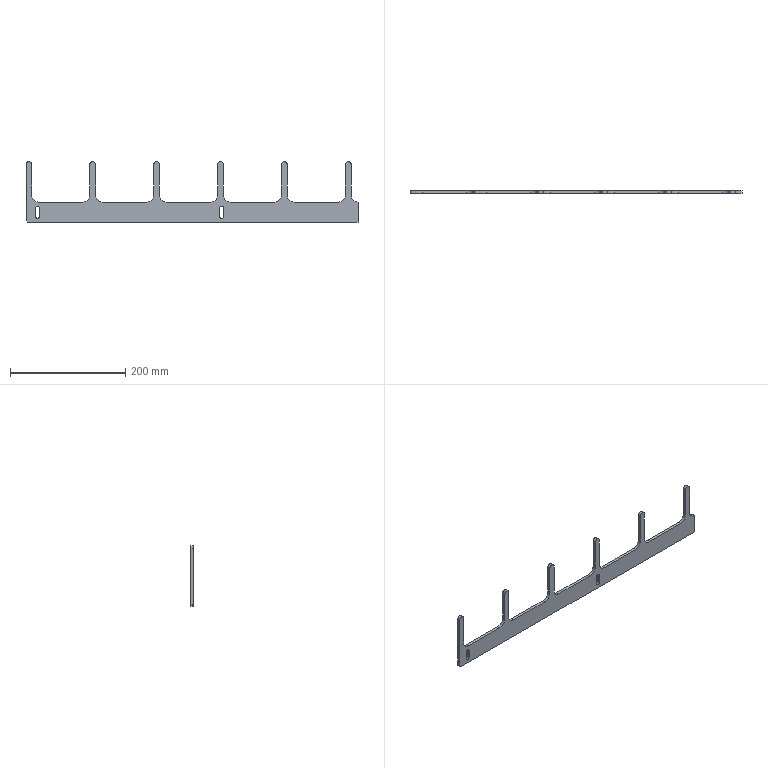Part | SolidWorks | features BaseBody 1, ICE 1 | 1 solid | 47 faces | box 577 x 5 x 105 mm | volume 122030 mm3 | plane 26 | cylinder 21 | commonest cylinder face diameters 24 x11 10 x6 6.5 x4
STEP:
#1=CARTESIAN_POINT('',(17.,0.,-5.));
#2=VERTEX_POINT('',#1);
#3=CARTESIAN_POINT('',(17.,0.,30.));
#4=VERTEX_POINT('',#3);
#5=CARTESIAN_POINT('',(17.,0.,47.5));
#6=DIRECTION('',(0.,0.,1.));
#7=VECTOR('',#6,1000.);
#8=LINE('',#5,#7);
#9=EDGE_CURVE('',#2,#4,#8,.T.);
#10=ORIENTED_EDGE('',*,*,#9,.F.);
#11=CARTESIAN_POINT('',(-557.5,0.,-5.));
#12=VERTEX_POINT('',#11);
#13=CARTESIAN_POINT('',(-557.5,0.,-5.));
#14=DIRECTION('',(1.,0.,0.));
#15=VECTOR('',#14,1000.);
#16=LINE('',#13,#15);
#17=EDGE_CURVE('',#12,#2,#16,.T.);
#18=ORIENTED_EDGE('',*,*,#17,.F.);
#19=CARTESIAN_POINT('',(-560.,0.,-2.5));
#20=VERTEX_POINT('',#19);
#21=CARTESIAN_POINT('',(-560.,0.,-2.5));
#22=DIRECTION('',(0.7071,0.,-0.7071));
#23=VECTOR('',#22,1000.);
#24=LINE('',#21,#23);
#25=EDGE_CURVE('',#20,#12,#24,.T.);
#26=ORIENTED_EDGE('',*,*,#25,.F.);
#27=CARTESIAN_POINT('',(-560.,0.,95.));
#28=VERTEX_POINT('',#27);
#29=CARTESIAN_POINT('',(-560.,0.,95.));
#30=DIRECTION('',(0.,0.,-1.));
#31=VECTOR('',#30,1000.);
#32=LINE('',#29,#31);
#33=EDGE_CURVE('',#28,#20,#32,.T.);
#34=ORIENTED_EDGE('',*,*,#33,.F.);
#35=CARTESIAN_POINT('',(-550.,0.,95.));
#36=VERTEX_POINT('',#35);
#37=CARTESIAN_POINT('',(-555.,0.,95.));
#38=DIRECTION('',(0.,-1.,0.));
#39=DIRECTION('',(1.,0.,0.));
#40=AXIS2_PLACEMENT_3D('',#37,#38,#39);
#41=CIRCLE('',#40,5.);
#42=EDGE_CURVE('',#36,#28,#41,.T.);
#43=ORIENTED_EDGE('',*,*,#42,.F.);
#44=CARTESIAN_POINT('',(-550.,0.,42.));
#45=VERTEX_POINT('',#44);
#46=CARTESIAN_POINT('',(-550.,0.,42.));
#47=DIRECTION('',(0.,0.,1.));
#48=VECTOR('',#47,1000.);
#49=LINE('',#46,#48);
#50=EDGE_CURVE('',#45,#36,#49,.T.);
#51=ORIENTED_EDGE('',*,*,#50,.F.);
#52=CARTESIAN_POINT('',(-538.,0.,30.));
#53=VERTEX_POINT('',#52);
#54=CARTESIAN_POINT('',(-538.,0.,42.));
#55=DIRECTION('',(0.,1.,0.));
#56=DIRECTION('',(0.,0.,-1.));
#57=AXIS2_PLACEMENT_3D('',#54,#55,#56);
#58=CIRCLE('',#57,12.);
#59=EDGE_CURVE('',#53,#45,#58,.T.);
#60=ORIENTED_EDGE('',*,*,#59,.F.);
#61=CARTESIAN_POINT('',(-461.,0.,30.));
#62=VERTEX_POINT('',#61);
#63=CARTESIAN_POINT('',(-461.,0.,30.));
#64=DIRECTION('',(-1.,0.,0.));
#65=VECTOR('',#64,1000.);
#66=LINE('',#63,#65);
#67=EDGE_CURVE('',#62,#53,#66,.T.);
#68=ORIENTED_EDGE('',*,*,#67,.F.);
#69=CARTESIAN_POINT('',(-449.,0.,42.));
#70=VERTEX_POINT('',#69);
#71=CARTESIAN_POINT('',(-461.,0.,42.));
#72=DIRECTION('',(0.,1.,0.));
#73=DIRECTION('',(1.,0.,0.));
#74=AXIS2_PLACEMENT_3D('',#71,#72,#73);
#75=CIRCLE('',#74,12.);
#76=EDGE_CURVE('',#70,#62,#75,.T.);
#77=ORIENTED_EDGE('',*,*,#76,.F.);
#78=CARTESIAN_POINT('',(-449.,0.,95.));
#79=VERTEX_POINT('',#78);
#80=CARTESIAN_POINT('',(-449.,0.,95.));
#81=DIRECTION('',(0.,0.,-1.));
#82=VECTOR('',#81,1000.);
#83=LINE('',#80,#82);
#84=EDGE_CURVE('',#79,#70,#83,.T.);
#85=ORIENTED_EDGE('',*,*,#84,.F.);
#86=CARTESIAN_POINT('',(-439.,0.,95.));
#87=VERTEX_POINT('',#86);
#88=CARTESIAN_POINT('',(-444.,0.,95.));
#89=DIRECTION('',(0.,-1.,0.));
#90=DIRECTION('',(1.,0.,0.));
#91=AXIS2_PLACEMENT_3D('',#88,#89,#90);
#92=CIRCLE('',#91,5.);
#93=EDGE_CURVE('',#87,#79,#92,.T.);
#94=ORIENTED_EDGE('',*,*,#93,.F.);
#95=CARTESIAN_POINT('',(-439.,0.,42.));
#96=VERTEX_POINT('',#95);
#97=CARTESIAN_POINT('',(-439.,0.,42.));
#98=DIRECTION('',(0.,0.,1.));
#99=VECTOR('',#98,1000.);
#100=LINE('',#97,#99);
#101=EDGE_CURVE('',#96,#87,#100,.T.);
#102=ORIENTED_EDGE('',*,*,#101,.F.);
#103=CARTESIAN_POINT('',(-427.,0.,30.));
#104=VERTEX_POINT('',#103);
#105=CARTESIAN_POINT('',(-427.,0.,42.));
#106=DIRECTION('',(0.,1.,0.));
#107=DIRECTION('',(0.,0.,-1.));
#108=AXIS2_PLACEMENT_3D('',#105,#106,#107);
#109=CIRCLE('',#108,12.);
#110=EDGE_CURVE('',#104,#96,#109,.T.);
#111=ORIENTED_EDGE('',*,*,#110,.F.);
#112=CARTESIAN_POINT('',(-350.,0.,30.));
#113=VERTEX_POINT('',#112);
#114=CARTESIAN_POINT('',(-350.,0.,30.));
#115=DIRECTION('',(-1.,0.,0.));
#116=VECTOR('',#115,1000.);
#117=LINE('',#114,#116);
#118=EDGE_CURVE('',#113,#104,#117,.T.);
#119=ORIENTED_EDGE('',*,*,#118,.F.);
#120=CARTESIAN_POINT('',(-338.,0.,42.));
#121=VERTEX_POINT('',#120);
#122=CARTESIAN_POINT('',(-350.,0.,42.));
#123=DIRECTION('',(0.,1.,0.));
#124=DIRECTION('',(1.,0.,0.));
#125=AXIS2_PLACEMENT_3D('',#122,#123,#124);
#126=CIRCLE('',#125,12.);
#127=EDGE_CURVE('',#121,#113,#126,.T.);
#128=ORIENTED_EDGE('',*,*,#127,.F.);
#129=CARTESIAN_POINT('',(-338.,0.,95.));
#130=VERTEX_POINT('',#129);
#131=CARTESIAN_POINT('',(-338.,0.,95.));
#132=DIRECTION('',(0.,0.,-1.));
#133=VECTOR('',#132,1000.);
#134=LINE('',#131,#133);
#135=EDGE_CURVE('',#130,#121,#134,.T.);
#136=ORIENTED_EDGE('',*,*,#135,.F.);
#137=CARTESIAN_POINT('',(-328.,0.,95.));
#138=VERTEX_POINT('',#137);
#139=CARTESIAN_POINT('',(-333.,0.,95.));
#140=DIRECTION('',(0.,-1.,0.));
#141=DIRECTION('',(1.,0.,0.));
#142=AXIS2_PLACEMENT_3D('',#139,#140,#141);
#143=CIRCLE('',#142,5.);
#144=EDGE_CURVE('',#138,#130,#143,.T.);
#145=ORIENTED_EDGE('',*,*,#144,.F.);
#146=CARTESIAN_POINT('',(-328.,0.,42.));
#147=VERTEX_POINT('',#146);
#148=CARTESIAN_POINT('',(-328.,0.,42.));
#149=DIRECTION('',(0.,0.,1.));
#150=VECTOR('',#149,1000.);
#151=LINE('',#148,#150);
#152=EDGE_CURVE('',#147,#138,#151,.T.);
#153=ORIENTED_EDGE('',*,*,#152,.F.);
#154=CARTESIAN_POINT('',(-316.,0.,30.));
#155=VERTEX_POINT('',#154);
#156=CARTESIAN_POINT('',(-316.,0.,42.));
#157=DIRECTION('',(0.,1.,0.));
#158=DIRECTION('',(0.,0.,-1.));
#159=AXIS2_PLACEMENT_3D('',#156,#157,#158);
#160=CIRCLE('',#159,12.);
#161=EDGE_CURVE('',#155,#147,#160,.T.);
#162=ORIENTED_EDGE('',*,*,#161,.F.);
#163=CARTESIAN_POINT('',(-239.,0.,30.));
#164=VERTEX_POINT('',#163);
#165=CARTESIAN_POINT('',(-239.,0.,30.));
#166=DIRECTION('',(-1.,0.,0.));
#167=VECTOR('',#166,1000.);
#168=LINE('',#165,#167);
#169=EDGE_CURVE('',#164,#155,#168,.T.);
#170=ORIENTED_EDGE('',*,*,#169,.F.);
#171=CARTESIAN_POINT('',(-227.,0.,42.));
#172=VERTEX_POINT('',#171);
#173=CARTESIAN_POINT('',(-239.,0.,42.));
#174=DIRECTION('',(0.,1.,0.));
#175=DIRECTION('',(1.,0.,0.));
#176=AXIS2_PLACEMENT_3D('',#173,#174,#175);
#177=CIRCLE('',#176,12.);
#178=EDGE_CURVE('',#172,#164,#177,.T.);
#179=ORIENTED_EDGE('',*,*,#178,.F.);
#180=CARTESIAN_POINT('',(-227.,0.,95.));
#181=VERTEX_POINT('',#180);
#182=CARTESIAN_POINT('',(-227.,0.,95.));
#183=DIRECTION('',(0.,0.,-1.));
#184=VECTOR('',#183,1000.);
#185=LINE('',#182,#184);
#186=EDGE_CURVE('',#181,#172,#185,.T.);
#187=ORIENTED_EDGE('',*,*,#186,.F.);
#188=CARTESIAN_POINT('',(-217.,0.,95.));
#189=VERTEX_POINT('',#188);
#190=CARTESIAN_POINT('',(-222.,0.,95.));
#191=DIRECTION('',(0.,-1.,0.));
#192=DIRECTION('',(1.,0.,0.));
#193=AXIS2_PLACEMENT_3D('',#190,#191,#192);
#194=CIRCLE('',#193,5.);
#195=EDGE_CURVE('',#189,#181,#194,.T.);
#196=ORIENTED_EDGE('',*,*,#195,.F.);
#197=CARTESIAN_POINT('',(-217.,0.,42.));
#198=VERTEX_POINT('',#197);
#199=CARTESIAN_POINT('',(-217.,0.,42.));
#200=DIRECTION('',(0.,0.,1.));
#201=VECTOR('',#200,1000.);
#202=LINE('',#199,#201);
#203=EDGE_CURVE('',#198,#189,#202,.T.);
#204=ORIENTED_EDGE('',*,*,#203,.F.);
#205=CARTESIAN_POINT('',(-205.,0.,30.));
#206=VERTEX_POINT('',#205);
#207=CARTESIAN_POINT('',(-205.,0.,42.));
#208=DIRECTION('',(0.,1.,0.));
#209=DIRECTION('',(0.,0.,-1.));
#210=AXIS2_PLACEMENT_3D('',#207,#208,#209);
#211=CIRCLE('',#210,12.);
#212=EDGE_CURVE('',#206,#198,#211,.T.);
#213=ORIENTED_EDGE('',*,*,#212,.F.);
#214=CARTESIAN_POINT('',(-128.,0.,30.));
#215=VERTEX_POINT('',#214);
#216=CARTESIAN_POINT('',(-128.,0.,30.));
#217=DIRECTION('',(-1.,0.,0.));
#218=VECTOR('',#217,1000.);
#219=LINE('',#216,#218);
#220=EDGE_CURVE('',#215,#206,#219,.T.);
#221=ORIENTED_EDGE('',*,*,#220,.F.);
#222=CARTESIAN_POINT('',(-116.,0.,42.));
#223=VERTEX_POINT('',#222);
#224=CARTESIAN_POINT('',(-128.,0.,42.));
#225=DIRECTION('',(0.,1.,0.));
#226=DIRECTION('',(1.,0.,0.));
#227=AXIS2_PLACEMENT_3D('',#224,#225,#226);
#228=CIRCLE('',#227,12.);
#229=EDGE_CURVE('',#223,#215,#228,.T.);
#230=ORIENTED_EDGE('',*,*,#229,.F.);
#231=CARTESIAN_POINT('',(-116.,0.,95.));
#232=VERTEX_POINT('',#231);
#233=CARTESIAN_POINT('',(-116.,0.,95.));
#234=DIRECTION('',(0.,0.,-1.));
#235=VECTOR('',#234,1000.);
#236=LINE('',#233,#235);
#237=EDGE_CURVE('',#232,#223,#236,.T.);
#238=ORIENTED_EDGE('',*,*,#237,.F.);
#239=CARTESIAN_POINT('',(-106.,0.,95.));
#240=VERTEX_POINT('',#239);
#241=CARTESIAN_POINT('',(-111.,0.,95.));
#242=DIRECTION('',(0.,-1.,0.));
#243=DIRECTION('',(1.,0.,0.));
#244=AXIS2_PLACEMENT_3D('',#241,#242,#243);
#245=CIRCLE('',#244,5.);
#246=EDGE_CURVE('',#240,#232,#245,.T.);
#247=ORIENTED_EDGE('',*,*,#246,.F.);
#248=CARTESIAN_POINT('',(-106.,0.,42.));
#249=VERTEX_POINT('',#248);
#250=CARTESIAN_POINT('',(-106.,0.,42.));
#251=DIRECTION('',(0.,0.,1.));
#252=VECTOR('',#251,1000.);
#253=LINE('',#250,#252);
#254=EDGE_CURVE('',#249,#240,#253,.T.);
#255=ORIENTED_EDGE('',*,*,#254,.F.);
#256=CARTESIAN_POINT('',(-94.,0.,30.));
#257=VERTEX_POINT('',#256);
#258=CARTESIAN_POINT('',(-94.,0.,42.));
#259=DIRECTION('',(0.,1.,0.));
#260=DIRECTION('',(0.,0.,-1.));
#261=AXIS2_PLACEMENT_3D('',#258,#259,#260);
#262=CIRCLE('',#261,12.);
#263=EDGE_CURVE('',#257,#249,#262,.T.);
#264=ORIENTED_EDGE('',*,*,#263,.F.);
#265=CARTESIAN_POINT('',(-17.,0.,30.));
#266=VERTEX_POINT('',#265);
#267=CARTESIAN_POINT('',(-17.,0.,30.));
#268=DIRECTION('',(-1.,0.,0.));
#269=VECTOR('',#268,1000.);
#270=LINE('',#267,#269);
#271=EDGE_CURVE('',#266,#257,#270,.T.);
#272=ORIENTED_EDGE('',*,*,#271,.F.);
#273=CARTESIAN_POINT('',(-5.,0.,42.));
#274=VERTEX_POINT('',#273);
#275=CARTESIAN_POINT('',(-17.,0.,42.));
#276=DIRECTION('',(0.,1.,0.));
#277=DIRECTION('',(1.,0.,0.));
#278=AXIS2_PLACEMENT_3D('',#275,#276,#277);
#279=CIRCLE('',#278,12.);
#280=EDGE_CURVE('',#274,#266,#279,.T.);
#281=ORIENTED_EDGE('',*,*,#280,.F.);
#282=CARTESIAN_POINT('',(-5.,0.,95.));
#283=VERTEX_POINT('',#282);
#284=CARTESIAN_POINT('',(-5.,0.,95.));
#285=DIRECTION('',(0.,0.,-1.));
#286=VECTOR('',#285,1000.);
#287=LINE('',#284,#286);
#288=EDGE_CURVE('',#283,#274,#287,.T.);
#289=ORIENTED_EDGE('',*,*,#288,.F.);
#290=CARTESIAN_POINT('',(5.,0.,95.));
#291=VERTEX_POINT('',#290);
#292=CARTESIAN_POINT('',(0.,0.,95.));
#293=DIRECTION('',(0.,-1.,0.));
#294=DIRECTION('',(1.,0.,0.));
#295=AXIS2_PLACEMENT_3D('',#292,#293,#294);
#296=CIRCLE('',#295,5.);
#297=EDGE_CURVE('',#291,#283,#296,.T.);
#298=ORIENTED_EDGE('',*,*,#297,.F.);
#299=CARTESIAN_POINT('',(5.,0.,42.));
#300=VERTEX_POINT('',#299);
#301=CARTESIAN_POINT('',(5.,0.,42.));
#302=DIRECTION('',(0.,0.,1.));
#303=VECTOR('',#302,1000.);
#304=LINE('',#301,#303);
#305=EDGE_CURVE('',#300,#291,#304,.T.);
#306=ORIENTED_EDGE('',*,*,#305,.F.);
#307=CARTESIAN_POINT('',(17.,0.,42.));
#308=DIRECTION('',(0.,1.,0.));
#309=DIRECTION('',(0.,0.,-1.));
#310=AXIS2_PLACEMENT_3D('',#307,#308,#309);
#311=CIRCLE('',#310,12.);
#312=EDGE_CURVE('',#4,#300,#311,.T.);
#313=ORIENTED_EDGE('',*,*,#312,.F.);
#314=EDGE_LOOP('',(#10,#18,#26,#34,#43,#51,#60,#68,#77,#85,#94,#102,#111,#119,#128,#136,#145,#153,#162,#170,#179,#187,#196,#204,#213,#221,#230,#238,#247,#255,#264,#272,#281,#289,#298,#306,#313));
#315=FACE_OUTER_BOUND('',#314,.T.);
#316=CARTESIAN_POINT('',(-223.25,0.,19.5));
#317=VERTEX_POINT('',#316);
#318=CARTESIAN_POINT('',(-216.75,0.,19.5));
#319=VERTEX_POINT('',#318);
#320=CARTESIAN_POINT('',(-220.,0.,19.5));
#321=DIRECTION('',(0.,1.,0.));
#322=DIRECTION('',(-1.,0.,0.));
#323=AXIS2_PLACEMENT_3D('',#320,#321,#322);
#324=CIRCLE('',#323,3.25);
#325=EDGE_CURVE('',#317,#319,#324,.T.);
#326=ORIENTED_EDGE('',*,*,#325,.F.);
#327=CARTESIAN_POINT('',(-223.25,0.,4.5));
#328=VERTEX_POINT('',#327);
#329=CARTESIAN_POINT('',(-223.25,0.,4.5));
#330=DIRECTION('',(0.,0.,1.));
#331=VECTOR('',#330,1000.);
#332=LINE('',#329,#331);
#333=EDGE_CURVE('',#328,#317,#332,.T.);
#334=ORIENTED_EDGE('',*,*,#333,.F.);
#335=CARTESIAN_POINT('',(-216.75,0.,4.5));
#336=VERTEX_POINT('',#335);
#337=CARTESIAN_POINT('',(-220.,0.,4.5));
#338=DIRECTION('',(0.,1.,0.));
#339=DIRECTION('',(1.,0.,0.));
#340=AXIS2_PLACEMENT_3D('',#337,#338,#339);
#341=CIRCLE('',#340,3.25);
#342=EDGE_CURVE('',#336,#328,#341,.T.);
#343=ORIENTED_EDGE('',*,*,#342,.F.);
#344=CARTESIAN_POINT('',(-216.75,0.,19.5));
#345=DIRECTION('',(0.,0.,-1.));
#346=VECTOR('',#345,1000.);
#347=LINE('',#344,#346);
#348=EDGE_CURVE('',#319,#336,#347,.T.);
#349=ORIENTED_EDGE('',*,*,#348,.F.);
#350=EDGE_LOOP('',(#326,#334,#343,#349));
#351=FACE_BOUND('',#350,.T.);
#352=CARTESIAN_POINT('',(-543.25,0.,4.5));
#353=VERTEX_POINT('',#352);
#354=CARTESIAN_POINT('',(-543.25,0.,19.5));
#355=VERTEX_POINT('',#354);
#356=CARTESIAN_POINT('',(-543.25,0.,4.5));
#357=DIRECTION('',(0.,0.,1.));
#358=VECTOR('',#357,1000.);
#359=LINE('',#356,#358);
#360=EDGE_CURVE('',#353,#355,#359,.T.);
#361=ORIENTED_EDGE('',*,*,#360,.F.);
#362=CARTESIAN_POINT('',(-536.75,0.,4.5));
#363=VERTEX_POINT('',#362);
#364=CARTESIAN_POINT('',(-540.,0.,4.5));
#365=DIRECTION('',(0.,1.,0.));
#366=DIRECTION('',(1.,0.,0.));
#367=AXIS2_PLACEMENT_3D('',#364,#365,#366);
#368=CIRCLE('',#367,3.25);
#369=EDGE_CURVE('',#363,#353,#368,.T.);
#370=ORIENTED_EDGE('',*,*,#369,.F.);
#371=CARTESIAN_POINT('',(-536.75,0.,19.5));
#372=VERTEX_POINT('',#371);
#373=CARTESIAN_POINT('',(-536.75,0.,19.5));
#374=DIRECTION('',(0.,0.,-1.));
#375=VECTOR('',#374,1000.);
#376=LINE('',#373,#375);
#377=EDGE_CURVE('',#372,#363,#376,.T.);
#378=ORIENTED_EDGE('',*,*,#377,.F.);
#379=CARTESIAN_POINT('',(-540.,0.,19.5));
#380=DIRECTION('',(0.,1.,0.));
#381=DIRECTION('',(-1.,0.,0.));
#382=AXIS2_PLACEMENT_3D('',#379,#380,#381);
#383=CIRCLE('',#382,3.25);
#384=EDGE_CURVE('',#355,#372,#383,.T.);
#385=ORIENTED_EDGE('',*,*,#384,.F.);
#386=EDGE_LOOP('',(#361,#370,#378,#385));
#387=FACE_BOUND('',#386,.T.);
#388=CARTESIAN_POINT('',(0.,0.,47.5));
#389=DIRECTION('',(0.,1.,0.));
#390=DIRECTION('',(0.,0.,-1.));
#391=AXIS2_PLACEMENT_3D('',#388,#389,#390);
#392=PLANE('',#391);
#393=ADVANCED_FACE('',(#315,#351,#387),#392,.T.);
#394=CARTESIAN_POINT('',(17.,-5.,30.));
#395=VERTEX_POINT('',#394);
#396=CARTESIAN_POINT('',(17.,-5.,-5.));
#397=VERTEX_POINT('',#396);
#398=CARTESIAN_POINT('',(17.,-5.,30.));
#399=DIRECTION('',(0.,0.,-1.));
#400=VECTOR('',#399,1000.);
#401=LINE('',#398,#400);
#402=EDGE_CURVE('',#395,#397,#401,.T.);
#403=ORIENTED_EDGE('',*,*,#402,.F.);
#404=CARTESIAN_POINT('',(5.,-5.,42.));
#405=VERTEX_POINT('',#404);
#406=CARTESIAN_POINT('',(17.,-5.,42.));
#407=DIRECTION('',(0.,-1.,0.));
#408=DIRECTION('',(-1.,0.,0.));
#409=AXIS2_PLACEMENT_3D('',#406,#407,#408);
#410=CIRCLE('',#409,12.);
#411=EDGE_CURVE('',#405,#395,#410,.T.);
#412=ORIENTED_EDGE('',*,*,#411,.F.);
#413=CARTESIAN_POINT('',(5.,-5.,95.));
#414=VERTEX_POINT('',#413);
#415=CARTESIAN_POINT('',(5.,-5.,95.));
#416=DIRECTION('',(0.,0.,-1.));
#417=VECTOR('',#416,1000.);
#418=LINE('',#415,#417);
#419=EDGE_CURVE('',#414,#405,#418,.T.);
#420=ORIENTED_EDGE('',*,*,#419,.F.);
#421=CARTESIAN_POINT('',(-5.,-5.,95.));
#422=VERTEX_POINT('',#421);
#423=CARTESIAN_POINT('',(0.,-5.,95.));
#424=DIRECTION('',(0.,1.,0.));
#425=DIRECTION('',(-1.,0.,0.));
#426=AXIS2_PLACEMENT_3D('',#423,#424,#425);
#427=CIRCLE('',#426,5.);
#428=EDGE_CURVE('',#422,#414,#427,.T.);
#429=ORIENTED_EDGE('',*,*,#428,.F.);
#430=CARTESIAN_POINT('',(-5.,-5.,42.));
#431=VERTEX_POINT('',#430);
#432=CARTESIAN_POINT('',(-5.,-5.,42.));
#433=DIRECTION('',(0.,0.,1.));
#434=VECTOR('',#433,1000.);
#435=LINE('',#432,#434);
#436=EDGE_CURVE('',#431,#422,#435,.T.);
#437=ORIENTED_EDGE('',*,*,#436,.F.);
#438=CARTESIAN_POINT('',(-17.,-5.,30.));
#439=VERTEX_POINT('',#438);
#440=CARTESIAN_POINT('',(-17.,-5.,42.));
#441=DIRECTION('',(0.,-1.,0.));
#442=DIRECTION('',(0.,0.,-1.));
#443=AXIS2_PLACEMENT_3D('',#440,#441,#442);
#444=CIRCLE('',#443,12.);
#445=EDGE_CURVE('',#439,#431,#444,.T.);
#446=ORIENTED_EDGE('',*,*,#445,.F.);
#447=CARTESIAN_POINT('',(-94.,-5.,30.));
#448=VERTEX_POINT('',#447);
#449=CARTESIAN_POINT('',(-94.,-5.,30.));
#450=DIRECTION('',(1.,0.,0.));
#451=VECTOR('',#450,1000.);
#452=LINE('',#449,#451);
#453=EDGE_CURVE('',#448,#439,#452,.T.);
#454=ORIENTED_EDGE('',*,*,#453,.F.);
#455=CARTESIAN_POINT('',(-106.,-5.,42.));
#456=VERTEX_POINT('',#455);
#457=CARTESIAN_POINT('',(-94.,-5.,42.));
#458=DIRECTION('',(0.,-1.,0.));
#459=DIRECTION('',(-1.,0.,0.));
#460=AXIS2_PLACEMENT_3D('',#457,#458,#459);
#461=CIRCLE('',#460,12.);
#462=EDGE_CURVE('',#456,#448,#461,.T.);
#463=ORIENTED_EDGE('',*,*,#462,.F.);
#464=CARTESIAN_POINT('',(-106.,-5.,95.));
#465=VERTEX_POINT('',#464);
#466=CARTESIAN_POINT('',(-106.,-5.,95.));
#467=DIRECTION('',(0.,0.,-1.));
#468=VECTOR('',#467,1000.);
#469=LINE('',#466,#468);
#470=EDGE_CURVE('',#465,#456,#469,.T.);
#471=ORIENTED_EDGE('',*,*,#470,.F.);
#472=CARTESIAN_POINT('',(-116.,-5.,95.));
#473=VERTEX_POINT('',#472);
#474=CARTESIAN_POINT('',(-111.,-5.,95.));
#475=DIRECTION('',(0.,1.,0.));
#476=DIRECTION('',(-1.,0.,0.));
#477=AXIS2_PLACEMENT_3D('',#474,#475,#476);
#478=CIRCLE('',#477,5.);
#479=EDGE_CURVE('',#473,#465,#478,.T.);
#480=ORIENTED_EDGE('',*,*,#479,.F.);
#481=CARTESIAN_POINT('',(-116.,-5.,42.));
#482=VERTEX_POINT('',#481);
#483=CARTESIAN_POINT('',(-116.,-5.,42.));
#484=DIRECTION('',(0.,0.,1.));
#485=VECTOR('',#484,1000.);
#486=LINE('',#483,#485);
#487=EDGE_CURVE('',#482,#473,#486,.T.);
#488=ORIENTED_EDGE('',*,*,#487,.F.);
#489=CARTESIAN_POINT('',(-128.,-5.,30.));
#490=VERTEX_POINT('',#489);
#491=CARTESIAN_POINT('',(-128.,-5.,42.));
#492=DIRECTION('',(0.,-1.,0.));
#493=DIRECTION('',(0.,0.,-1.));
#494=AXIS2_PLACEMENT_3D('',#491,#492,#493);
#495=CIRCLE('',#494,12.);
#496=EDGE_CURVE('',#490,#482,#495,.T.);
#497=ORIENTED_EDGE('',*,*,#496,.F.);
#498=CARTESIAN_POINT('',(-205.,-5.,30.));
#499=VERTEX_POINT('',#498);
#500=CARTESIAN_POINT('',(-205.,-5.,30.));
#501=DIRECTION('',(1.,0.,0.));
#502=VECTOR('',#501,1000.);
#503=LINE('',#500,#502);
#504=EDGE_CURVE('',#499,#490,#503,.T.);
#505=ORIENTED_EDGE('',*,*,#504,.F.);
#506=CARTESIAN_POINT('',(-217.,-5.,42.));
#507=VERTEX_POINT('',#506);
#508=CARTESIAN_POINT('',(-205.,-5.,42.));
#509=DIRECTION('',(0.,-1.,0.));
#510=DIRECTION('',(-1.,0.,0.));
#511=AXIS2_PLACEMENT_3D('',#508,#509,#510);
#512=CIRCLE('',#511,12.);
#513=EDGE_CURVE('',#507,#499,#512,.T.);
#514=ORIENTED_EDGE('',*,*,#513,.F.);
#515=CARTESIAN_POINT('',(-217.,-5.,95.));
#516=VERTEX_POINT('',#515);
#517=CARTESIAN_POINT('',(-217.,-5.,95.));
#518=DIRECTION('',(0.,0.,-1.));
#519=VECTOR('',#518,1000.);
#520=LINE('',#517,#519);
#521=EDGE_CURVE('',#516,#507,#520,.T.);
#522=ORIENTED_EDGE('',*,*,#521,.F.);
#523=CARTESIAN_POINT('',(-227.,-5.,95.));
#524=VERTEX_POINT('',#523);
#525=CARTESIAN_POINT('',(-222.,-5.,95.));
#526=DIRECTION('',(0.,1.,0.));
#527=DIRECTION('',(-1.,0.,0.));
#528=AXIS2_PLACEMENT_3D('',#525,#526,#527);
#529=CIRCLE('',#528,5.);
#530=EDGE_CURVE('',#524,#516,#529,.T.);
#531=ORIENTED_EDGE('',*,*,#530,.F.);
#532=CARTESIAN_POINT('',(-227.,-5.,42.));
#533=VERTEX_POINT('',#532);
#534=CARTESIAN_POINT('',(-227.,-5.,42.));
#535=DIRECTION('',(0.,0.,1.));
#536=VECTOR('',#535,1000.);
#537=LINE('',#534,#536);
#538=EDGE_CURVE('',#533,#524,#537,.T.);
#539=ORIENTED_EDGE('',*,*,#538,.F.);
#540=CARTESIAN_POINT('',(-239.,-5.,30.));
#541=VERTEX_POINT('',#540);
#542=CARTESIAN_POINT('',(-239.,-5.,42.));
#543=DIRECTION('',(0.,-1.,0.));
#544=DIRECTION('',(0.,0.,-1.));
#545=AXIS2_PLACEMENT_3D('',#542,#543,#544);
#546=CIRCLE('',#545,12.);
#547=EDGE_CURVE('',#541,#533,#546,.T.);
#548=ORIENTED_EDGE('',*,*,#547,.F.);
#549=CARTESIAN_POINT('',(-316.,-5.,30.));
#550=VERTEX_POINT('',#549);
#551=CARTESIAN_POINT('',(-316.,-5.,30.));
#552=DIRECTION('',(1.,0.,0.));
#553=VECTOR('',#552,1000.);
#554=LINE('',#551,#553);
#555=EDGE_CURVE('',#550,#541,#554,.T.);
#556=ORIENTED_EDGE('',*,*,#555,.F.);
#557=CARTESIAN_POINT('',(-328.,-5.,42.));
#558=VERTEX_POINT('',#557);
#559=CARTESIAN_POINT('',(-316.,-5.,42.));
#560=DIRECTION('',(0.,-1.,0.));
#561=DIRECTION('',(-1.,0.,0.));
#562=AXIS2_PLACEMENT_3D('',#559,#560,#561);
#563=CIRCLE('',#562,12.);
#564=EDGE_CURVE('',#558,#550,#563,.T.);
#565=ORIENTED_EDGE('',*,*,#564,.F.);
#566=CARTESIAN_POINT('',(-328.,-5.,95.));
#567=VERTEX_POINT('',#566);
#568=CARTESIAN_POINT('',(-328.,-5.,95.));
#569=DIRECTION('',(0.,0.,-1.));
#570=VECTOR('',#569,1000.);
#571=LINE('',#568,#570);
#572=EDGE_CURVE('',#567,#558,#571,.T.);
#573=ORIENTED_EDGE('',*,*,#572,.F.);
#574=CARTESIAN_POINT('',(-338.,-5.,95.));
#575=VERTEX_POINT('',#574);
#576=CARTESIAN_POINT('',(-333.,-5.,95.));
#577=DIRECTION('',(0.,1.,0.));
#578=DIRECTION('',(-1.,0.,0.));
#579=AXIS2_PLACEMENT_3D('',#576,#577,#578);
#580=CIRCLE('',#579,5.);
#581=EDGE_CURVE('',#575,#567,#580,.T.);
#582=ORIENTED_EDGE('',*,*,#581,.F.);
#583=CARTESIAN_POINT('',(-338.,-5.,42.));
#584=VERTEX_POINT('',#583);
#585=CARTESIAN_POINT('',(-338.,-5.,42.));
#586=DIRECTION('',(0.,0.,1.));
#587=VECTOR('',#586,1000.);
#588=LINE('',#585,#587);
#589=EDGE_CURVE('',#584,#575,#588,.T.);
#590=ORIENTED_EDGE('',*,*,#589,.F.);
#591=CARTESIAN_POINT('',(-350.,-5.,30.));
#592=VERTEX_POINT('',#591);
#593=CARTESIAN_POINT('',(-350.,-5.,42.));
#594=DIRECTION('',(0.,-1.,0.));
#595=DIRECTION('',(0.,0.,-1.));
#596=AXIS2_PLACEMENT_3D('',#593,#594,#595);
#597=CIRCLE('',#596,12.);
#598=EDGE_CURVE('',#592,#584,#597,.T.);
#599=ORIENTED_EDGE('',*,*,#598,.F.);
#600=CARTESIAN_POINT('',(-427.,-5.,30.));
#601=VERTEX_POINT('',#600);
#602=CARTESIAN_POINT('',(-427.,-5.,30.));
#603=DIRECTION('',(1.,0.,0.));
#604=VECTOR('',#603,1000.);
#605=LINE('',#602,#604);
#606=EDGE_CURVE('',#601,#592,#605,.T.);
#607=ORIENTED_EDGE('',*,*,#606,.F.);
#608=CARTESIAN_POINT('',(-439.,-5.,42.));
#609=VERTEX_POINT('',#608);
#610=CARTESIAN_POINT('',(-427.,-5.,42.));
#611=DIRECTION('',(0.,-1.,0.));
#612=DIRECTION('',(-1.,0.,0.));
#613=AXIS2_PLACEMENT_3D('',#610,#611,#612);
#614=CIRCLE('',#613,12.);
#615=EDGE_CURVE('',#609,#601,#614,.T.);
#616=ORIENTED_EDGE('',*,*,#615,.F.);
#617=CARTESIAN_POINT('',(-439.,-5.,95.));
#618=VERTEX_POINT('',#617);
#619=CARTESIAN_POINT('',(-439.,-5.,95.));
#620=DIRECTION('',(0.,0.,-1.));
#621=VECTOR('',#620,1000.);
#622=LINE('',#619,#621);
#623=EDGE_CURVE('',#618,#609,#622,.T.);
#624=ORIENTED_EDGE('',*,*,#623,.F.);
#625=CARTESIAN_POINT('',(-449.,-5.,95.));
#626=VERTEX_POINT('',#625);
#627=CARTESIAN_POINT('',(-444.,-5.,95.));
#628=DIRECTION('',(0.,1.,0.));
#629=DIRECTION('',(-1.,0.,0.));
#630=AXIS2_PLACEMENT_3D('',#627,#628,#629);
#631=CIRCLE('',#630,5.);
#632=EDGE_CURVE('',#626,#618,#631,.T.);
#633=ORIENTED_EDGE('',*,*,#632,.F.);
#634=CARTESIAN_POINT('',(-449.,-5.,42.));
#635=VERTEX_POINT('',#634);
#636=CARTESIAN_POINT('',(-449.,-5.,42.));
#637=DIRECTION('',(0.,0.,1.));
#638=VECTOR('',#637,1000.);
#639=LINE('',#636,#638);
#640=EDGE_CURVE('',#635,#626,#639,.T.);
#641=ORIENTED_EDGE('',*,*,#640,.F.);
#642=CARTESIAN_POINT('',(-461.,-5.,30.));
#643=VERTEX_POINT('',#642);
#644=CARTESIAN_POINT('',(-461.,-5.,42.));
#645=DIRECTION('',(0.,-1.,0.));
#646=DIRECTION('',(0.,0.,-1.));
#647=AXIS2_PLACEMENT_3D('',#644,#645,#646);
#648=CIRCLE('',#647,12.);
#649=EDGE_CURVE('',#643,#635,#648,.T.);
#650=ORIENTED_EDGE('',*,*,#649,.F.);
#651=CARTESIAN_POINT('',(-538.,-5.,30.));
#652=VERTEX_POINT('',#651);
#653=CARTESIAN_POINT('',(-538.,-5.,30.));
#654=DIRECTION('',(1.,0.,0.));
#655=VECTOR('',#654,1000.);
#656=LINE('',#653,#655);
#657=EDGE_CURVE('',#652,#643,#656,.T.);
#658=ORIENTED_EDGE('',*,*,#657,.F.);
#659=CARTESIAN_POINT('',(-550.,-5.,42.));
#660=VERTEX_POINT('',#659);
#661=CARTESIAN_POINT('',(-538.,-5.,42.));
#662=DIRECTION('',(0.,-1.,0.));
#663=DIRECTION('',(-1.,0.,0.));
#664=AXIS2_PLACEMENT_3D('',#661,#662,#663);
#665=CIRCLE('',#664,12.);
#666=EDGE_CURVE('',#660,#652,#665,.T.);
#667=ORIENTED_EDGE('',*,*,#666,.F.);
#668=CARTESIAN_POINT('',(-550.,-5.,95.));
#669=VERTEX_POINT('',#668);
#670=CARTESIAN_POINT('',(-550.,-5.,95.));
#671=DIRECTION('',(0.,0.,-1.));
#672=VECTOR('',#671,1000.);
#673=LINE('',#670,#672);
#674=EDGE_CURVE('',#669,#660,#673,.T.);
#675=ORIENTED_EDGE('',*,*,#674,.F.);
#676=CARTESIAN_POINT('',(-560.,-5.,95.));
#677=VERTEX_POINT('',#676);
#678=CARTESIAN_POINT('',(-555.,-5.,95.));
#679=DIRECTION('',(0.,1.,0.));
#680=DIRECTION('',(-1.,0.,0.));
#681=AXIS2_PLACEMENT_3D('',#678,#679,#680);
#682=CIRCLE('',#681,5.);
#683=EDGE_CURVE('',#677,#669,#682,.T.);
#684=ORIENTED_EDGE('',*,*,#683,.F.);
#685=CARTESIAN_POINT('',(-560.,-5.,-2.5));
#686=VERTEX_POINT('',#685);
#687=CARTESIAN_POINT('',(-560.,-5.,-2.5));
#688=DIRECTION('',(0.,0.,1.));
#689=VECTOR('',#688,1000.);
#690=LINE('',#687,#689);
#691=EDGE_CURVE('',#686,#677,#690,.T.);
#692=ORIENTED_EDGE('',*,*,#691,.F.);
#693=CARTESIAN_POINT('',(-557.5,-5.,-5.));
#694=VERTEX_POINT('',#693);
#695=CARTESIAN_POINT('',(-557.5,-5.,-5.));
#696=DIRECTION('',(-0.7071,0.,0.7071));
#697=VECTOR('',#696,1000.);
#698=LINE('',#695,#697);
#699=EDGE_CURVE('',#694,#686,#698,.T.);
#700=ORIENTED_EDGE('',*,*,#699,.F.);
#701=CARTESIAN_POINT('',(557.5,-5.,-5.));
#702=DIRECTION('',(-1.,0.,0.));
#703=VECTOR('',#702,1000.);
#704=LINE('',#701,#703);
#705=EDGE_CURVE('',#397,#694,#704,.T.);
#706=ORIENTED_EDGE('',*,*,#705,.F.);
#707=EDGE_LOOP('',(#403,#412,#420,#429,#437,#446,#454,#463,#471,#480,#488,#497,#505,#514,#522,#531,#539,#548,#556,#565,#573,#582,#590,#599,#607,#616,#624,#633,#641,#650,#658,#667,#675,#684,#692,#700,#706));
#708=FACE_OUTER_BOUND('',#707,.T.);
#709=CARTESIAN_POINT('',(-216.75,-5.,19.5));
#710=VERTEX_POINT('',#709);
#711=CARTESIAN_POINT('',(-223.25,-5.,19.5));
#712=VERTEX_POINT('',#711);
#713=CARTESIAN_POINT('',(-220.,-5.,19.5));
#714=DIRECTION('',(0.,-1.,0.));
#715=DIRECTION('',(1.,0.,0.));
#716=AXIS2_PLACEMENT_3D('',#713,#714,#715);
#717=CIRCLE('',#716,3.25);
#718=EDGE_CURVE('',#710,#712,#717,.T.);
#719=ORIENTED_EDGE('',*,*,#718,.F.);
#720=CARTESIAN_POINT('',(-216.75,-5.,4.5));
#721=VERTEX_POINT('',#720);
#722=CARTESIAN_POINT('',(-216.75,-5.,4.5));
#723=DIRECTION('',(0.,0.,1.));
#724=VECTOR('',#723,1000.);
#725=LINE('',#722,#724);
#726=EDGE_CURVE('',#721,#710,#725,.T.);
#727=ORIENTED_EDGE('',*,*,#726,.F.);
#728=CARTESIAN_POINT('',(-223.25,-5.,4.5));
#729=VERTEX_POINT('',#728);
#730=CARTESIAN_POINT('',(-220.,-5.,4.5));
#731=DIRECTION('',(0.,-1.,0.));
#732=DIRECTION('',(-1.,0.,0.));
#733=AXIS2_PLACEMENT_3D('',#730,#731,#732);
#734=CIRCLE('',#733,3.25);
#735=EDGE_CURVE('',#729,#721,#734,.T.);
#736=ORIENTED_EDGE('',*,*,#735,.F.);
#737=CARTESIAN_POINT('',(-223.25,-5.,19.5));
#738=DIRECTION('',(0.,0.,-1.));
#739=VECTOR('',#738,1000.);
#740=LINE('',#737,#739);
#741=EDGE_CURVE('',#712,#729,#740,.T.);
#742=ORIENTED_EDGE('',*,*,#741,.F.);
#743=EDGE_LOOP('',(#719,#727,#736,#742));
#744=FACE_BOUND('',#743,.T.);
#745=CARTESIAN_POINT('',(-543.25,-5.,19.5));
#746=VERTEX_POINT('',#745);
#747=CARTESIAN_POINT('',(-543.25,-5.,4.5));
#748=VERTEX_POINT('',#747);
#749=CARTESIAN_POINT('',(-543.25,-5.,19.5));
#750=DIRECTION('',(0.,0.,-1.));
#751=VECTOR('',#750,1000.);
#752=LINE('',#749,#751);
#753=EDGE_CURVE('',#746,#748,#752,.T.);
#754=ORIENTED_EDGE('',*,*,#753,.F.);
#755=CARTESIAN_POINT('',(-536.75,-5.,19.5));
#756=VERTEX_POINT('',#755);
#757=CARTESIAN_POINT('',(-540.,-5.,19.5));
#758=DIRECTION('',(0.,-1.,0.));
#759=DIRECTION('',(1.,0.,0.));
#760=AXIS2_PLACEMENT_3D('',#757,#758,#759);
#761=CIRCLE('',#760,3.25);
#762=EDGE_CURVE('',#756,#746,#761,.T.);
#763=ORIENTED_EDGE('',*,*,#762,.F.);
#764=CARTESIAN_POINT('',(-536.75,-5.,4.5));
#765=VERTEX_POINT('',#764);
#766=CARTESIAN_POINT('',(-536.75,-5.,4.5));
#767=DIRECTION('',(0.,0.,1.));
#768=VECTOR('',#767,1000.);
#769=LINE('',#766,#768);
#770=EDGE_CURVE('',#765,#756,#769,.T.);
#771=ORIENTED_EDGE('',*,*,#770,.F.);
#772=CARTESIAN_POINT('',(-540.,-5.,4.5));
#773=DIRECTION('',(0.,-1.,0.));
#774=DIRECTION('',(-1.,0.,0.));
#775=AXIS2_PLACEMENT_3D('',#772,#773,#774);
#776=CIRCLE('',#775,3.25);
#777=EDGE_CURVE('',#748,#765,#776,.T.);
#778=ORIENTED_EDGE('',*,*,#777,.F.);
#779=EDGE_LOOP('',(#754,#763,#771,#778));
#780=FACE_BOUND('',#779,.T.);
#781=CARTESIAN_POINT('',(0.,-5.,47.5));
#782=DIRECTION('',(0.,-1.,0.));
#783=DIRECTION('',(0.,0.,-1.));
#784=AXIS2_PLACEMENT_3D('',#781,#782,#783);
#785=PLANE('',#784);
#786=ADVANCED_FACE('',(#708,#744,#780),#785,.T.);
#787=ORIENTED_EDGE('',*,*,#152,.T.);
#788=CARTESIAN_POINT('',(-328.,-5.,95.));
#789=DIRECTION('',(0.,1.,0.));
#790=VECTOR('',#789,1000.);
#791=LINE('',#788,#790);
#792=EDGE_CURVE('',#567,#138,#791,.T.);
#793=ORIENTED_EDGE('',*,*,#792,.F.);
#794=ORIENTED_EDGE('',*,*,#572,.T.);
#795=CARTESIAN_POINT('',(-328.,0.,42.));
#796=DIRECTION('',(0.,-1.,0.));
#797=VECTOR('',#796,1000.);
#798=LINE('',#795,#797);
#799=EDGE_CURVE('',#147,#558,#798,.T.);
#800=ORIENTED_EDGE('',*,*,#799,.F.);
#801=EDGE_LOOP('',(#787,#793,#794,#800));
#802=FACE_OUTER_BOUND('',#801,.T.);
#803=CARTESIAN_POINT('',(-328.,0.,42.));
#804=DIRECTION('',(1.,0.,0.));
#805=DIRECTION('',(0.,1.,0.));
#806=AXIS2_PLACEMENT_3D('',#803,#804,#805);
#807=PLANE('',#806);
#808=ADVANCED_FACE('',(#802),#807,.T.);
#809=ORIENTED_EDGE('',*,*,#144,.T.);
#810=CARTESIAN_POINT('',(-338.,-5.,95.));
#811=DIRECTION('',(0.,1.,0.));
#812=VECTOR('',#811,1000.);
#813=LINE('',#810,#812);
#814=EDGE_CURVE('',#575,#130,#813,.T.);
#815=ORIENTED_EDGE('',*,*,#814,.F.);
#816=ORIENTED_EDGE('',*,*,#581,.T.);
#817=ORIENTED_EDGE('',*,*,#792,.T.);
#818=EDGE_LOOP('',(#809,#815,#816,#817));
#819=FACE_OUTER_BOUND('',#818,.T.);
#820=CARTESIAN_POINT('',(-333.,0.,95.));
#821=DIRECTION('',(0.,-1.,0.));
#822=DIRECTION('',(-1.,0.,0.));
#823=AXIS2_PLACEMENT_3D('',#820,#821,#822);
#824=CYLINDRICAL_SURFACE('',#823,5.);
#825=ADVANCED_FACE('',(#819),#824,.T.);
#826=ORIENTED_EDGE('',*,*,#135,.T.);
#827=CARTESIAN_POINT('',(-338.,-5.,42.));
#828=DIRECTION('',(0.,1.,0.));
#829=VECTOR('',#828,1000.);
#830=LINE('',#827,#829);
#831=EDGE_CURVE('',#584,#121,#830,.T.);
#832=ORIENTED_EDGE('',*,*,#831,.F.);
#833=ORIENTED_EDGE('',*,*,#589,.T.);
#834=ORIENTED_EDGE('',*,*,#814,.T.);
#835=EDGE_LOOP('',(#826,#832,#833,#834));
#836=FACE_OUTER_BOUND('',#835,.T.);
#837=CARTESIAN_POINT('',(-338.,0.,95.));
#838=DIRECTION('',(-1.,0.,0.));
#839=DIRECTION('',(0.,0.,1.));
#840=AXIS2_PLACEMENT_3D('',#837,#838,#839);
#841=PLANE('',#840);
#842=ADVANCED_FACE('',(#836),#841,.T.);
#843=ORIENTED_EDGE('',*,*,#127,.T.);
#844=CARTESIAN_POINT('',(-350.,-5.,30.));
#845=DIRECTION('',(0.,1.,0.));
#846=VECTOR('',#845,1000.);
#847=LINE('',#844,#846);
#848=EDGE_CURVE('',#592,#113,#847,.T.);
#849=ORIENTED_EDGE('',*,*,#848,.F.);
#850=ORIENTED_EDGE('',*,*,#598,.T.);
#851=ORIENTED_EDGE('',*,*,#831,.T.);
#852=EDGE_LOOP('',(#843,#849,#850,#851));
#853=FACE_OUTER_BOUND('',#852,.T.);
#854=CARTESIAN_POINT('',(-350.,0.,42.));
#855=DIRECTION('',(0.,-1.,0.));
#856=DIRECTION('',(-0.000005163,0.,-1.));
#857=AXIS2_PLACEMENT_3D('',#854,#855,#856);
#858=CYLINDRICAL_SURFACE('',#857,12.);
#859=ADVANCED_FACE('',(#853),#858,.F.);
#860=ORIENTED_EDGE('',*,*,#118,.T.);
#861=CARTESIAN_POINT('',(-427.,-5.,30.));
#862=DIRECTION('',(0.,1.,0.));
#863=VECTOR('',#862,1000.);
#864=LINE('',#861,#863);
#865=EDGE_CURVE('',#601,#104,#864,.T.);
#866=ORIENTED_EDGE('',*,*,#865,.F.);
#867=ORIENTED_EDGE('',*,*,#606,.T.);
#868=ORIENTED_EDGE('',*,*,#848,.T.);
#869=EDGE_LOOP('',(#860,#866,#867,#868));
#870=FACE_OUTER_BOUND('',#869,.T.);
#871=CARTESIAN_POINT('',(-350.,0.,30.));
#872=DIRECTION('',(0.,0.,1.));
#873=DIRECTION('',(1.,0.,0.));
#874=AXIS2_PLACEMENT_3D('',#871,#872,#873);
#875=PLANE('',#874);
#876=ADVANCED_FACE('',(#870),#875,.T.);
#877=ORIENTED_EDGE('',*,*,#110,.T.);
#878=CARTESIAN_POINT('',(-439.,-5.,42.));
#879=DIRECTION('',(0.,1.,0.));
#880=VECTOR('',#879,1000.);
#881=LINE('',#878,#880);
#882=EDGE_CURVE('',#609,#96,#881,.T.);
#883=ORIENTED_EDGE('',*,*,#882,.F.);
#884=ORIENTED_EDGE('',*,*,#615,.T.);
#885=ORIENTED_EDGE('',*,*,#865,.T.);
#886=EDGE_LOOP('',(#877,#883,#884,#885));
#887=FACE_OUTER_BOUND('',#886,.T.);
#888=CARTESIAN_POINT('',(-427.,0.,42.));
#889=DIRECTION('',(0.,-1.,0.));
#890=DIRECTION('',(-1.,0.,0.000005163));
#891=AXIS2_PLACEMENT_3D('',#888,#889,#890);
#892=CYLINDRICAL_SURFACE('',#891,12.);
#893=ADVANCED_FACE('',(#887),#892,.F.);
#894=ORIENTED_EDGE('',*,*,#101,.T.);
#895=CARTESIAN_POINT('',(-439.,-5.,95.));
#896=DIRECTION('',(0.,1.,0.));
#897=VECTOR('',#896,1000.);
#898=LINE('',#895,#897);
#899=EDGE_CURVE('',#618,#87,#898,.T.);
#900=ORIENTED_EDGE('',*,*,#899,.F.);
#901=ORIENTED_EDGE('',*,*,#623,.T.);
#902=ORIENTED_EDGE('',*,*,#882,.T.);
#903=EDGE_LOOP('',(#894,#900,#901,#902));
#904=FACE_OUTER_BOUND('',#903,.T.);
#905=CARTESIAN_POINT('',(-439.,0.,42.));
#906=DIRECTION('',(1.,0.,0.));
#907=DIRECTION('',(0.,1.,0.));
#908=AXIS2_PLACEMENT_3D('',#905,#906,#907);
#909=PLANE('',#908);
#910=ADVANCED_FACE('',(#904),#909,.T.);
#911=ORIENTED_EDGE('',*,*,#93,.T.);
#912=CARTESIAN_POINT('',(-449.,-5.,95.));
#913=DIRECTION('',(0.,1.,0.));
#914=VECTOR('',#913,1000.);
#915=LINE('',#912,#914);
#916=EDGE_CURVE('',#626,#79,#915,.T.);
#917=ORIENTED_EDGE('',*,*,#916,.F.);
#918=ORIENTED_EDGE('',*,*,#632,.T.);
#919=ORIENTED_EDGE('',*,*,#899,.T.);
#920=EDGE_LOOP('',(#911,#917,#918,#919));
#921=FACE_OUTER_BOUND('',#920,.T.);
#922=CARTESIAN_POINT('',(-444.,0.,95.));
#923=DIRECTION('',(0.,-1.,0.));
#924=DIRECTION('',(-1.,0.,0.));
#925=AXIS2_PLACEMENT_3D('',#922,#923,#924);
#926=CYLINDRICAL_SURFACE('',#925,5.);
#927=ADVANCED_FACE('',(#921),#926,.T.);
#928=ORIENTED_EDGE('',*,*,#84,.T.);
#929=CARTESIAN_POINT('',(-449.,-5.,42.));
#930=DIRECTION('',(0.,1.,0.));
#931=VECTOR('',#930,1000.);
#932=LINE('',#929,#931);
#933=EDGE_CURVE('',#635,#70,#932,.T.);
#934=ORIENTED_EDGE('',*,*,#933,.F.);
#935=ORIENTED_EDGE('',*,*,#640,.T.);
#936=ORIENTED_EDGE('',*,*,#916,.T.);
#937=EDGE_LOOP('',(#928,#934,#935,#936));
#938=FACE_OUTER_BOUND('',#937,.T.);
#939=CARTESIAN_POINT('',(-449.,0.,95.));
#940=DIRECTION('',(-1.,0.,0.));
#941=DIRECTION('',(0.,0.,1.));
#942=AXIS2_PLACEMENT_3D('',#939,#940,#941);
#943=PLANE('',#942);
#944=ADVANCED_FACE('',(#938),#943,.T.);
#945=ORIENTED_EDGE('',*,*,#76,.T.);
#946=CARTESIAN_POINT('',(-461.,-5.,30.));
#947=DIRECTION('',(0.,1.,0.));
#948=VECTOR('',#947,1000.);
#949=LINE('',#946,#948);
#950=EDGE_CURVE('',#643,#62,#949,.T.);
#951=ORIENTED_EDGE('',*,*,#950,.F.);
#952=ORIENTED_EDGE('',*,*,#649,.T.);
#953=ORIENTED_EDGE('',*,*,#933,.T.);
#954=EDGE_LOOP('',(#945,#951,#952,#953));
#955=FACE_OUTER_BOUND('',#954,.T.);
#956=CARTESIAN_POINT('',(-461.,0.,42.));
#957=DIRECTION('',(0.,-1.,0.));
#958=DIRECTION('',(-0.000005163,0.,-1.));
#959=AXIS2_PLACEMENT_3D('',#956,#957,#958);
#960=CYLINDRICAL_SURFACE('',#959,12.);
#961=ADVANCED_FACE('',(#955),#960,.F.);
#962=ORIENTED_EDGE('',*,*,#67,.T.);
#963=CARTESIAN_POINT('',(-538.,-5.,30.));
#964=DIRECTION('',(0.,1.,0.));
#965=VECTOR('',#964,1000.);
#966=LINE('',#963,#965);
#967=EDGE_CURVE('',#652,#53,#966,.T.);
#968=ORIENTED_EDGE('',*,*,#967,.F.);
#969=ORIENTED_EDGE('',*,*,#657,.T.);
#970=ORIENTED_EDGE('',*,*,#950,.T.);
#971=EDGE_LOOP('',(#962,#968,#969,#970));
#972=FACE_OUTER_BOUND('',#971,.T.);
#973=CARTESIAN_POINT('',(-461.,0.,30.));
#974=DIRECTION('',(0.,0.,1.));
#975=DIRECTION('',(1.,0.,0.));
#976=AXIS2_PLACEMENT_3D('',#973,#974,#975);
#977=PLANE('',#976);
#978=ADVANCED_FACE('',(#972),#977,.T.);
#979=ORIENTED_EDGE('',*,*,#59,.T.);
#980=CARTESIAN_POINT('',(-550.,-5.,42.));
#981=DIRECTION('',(0.,1.,0.));
#982=VECTOR('',#981,1000.);
#983=LINE('',#980,#982);
#984=EDGE_CURVE('',#660,#45,#983,.T.);
#985=ORIENTED_EDGE('',*,*,#984,.F.);
#986=ORIENTED_EDGE('',*,*,#666,.T.);
#987=ORIENTED_EDGE('',*,*,#967,.T.);
#988=EDGE_LOOP('',(#979,#985,#986,#987));
#989=FACE_OUTER_BOUND('',#988,.T.);
#990=CARTESIAN_POINT('',(-538.,0.,42.));
#991=DIRECTION('',(0.,-1.,0.));
#992=DIRECTION('',(-1.,0.,0.000005163));
#993=AXIS2_PLACEMENT_3D('',#990,#991,#992);
#994=CYLINDRICAL_SURFACE('',#993,12.);
#995=ADVANCED_FACE('',(#989),#994,.F.);
#996=ORIENTED_EDGE('',*,*,#50,.T.);
#997=CARTESIAN_POINT('',(-550.,-5.,95.));
#998=DIRECTION('',(0.,1.,0.));
#999=VECTOR('',#998,1000.);
#1000=LINE('',#997,#999);
#1001=EDGE_CURVE('',#669,#36,#1000,.T.);
#1002=ORIENTED_EDGE('',*,*,#1001,.F.);
#1003=ORIENTED_EDGE('',*,*,#674,.T.);
#1004=ORIENTED_EDGE('',*,*,#984,.T.);
#1005=EDGE_LOOP('',(#996,#1002,#1003,#1004));
#1006=FACE_OUTER_BOUND('',#1005,.T.);
#1007=CARTESIAN_POINT('',(-550.,0.,42.));
#1008=DIRECTION('',(1.,0.,0.));
#1009=DIRECTION('',(0.,1.,0.));
#1010=AXIS2_PLACEMENT_3D('',#1007,#1008,#1009);
#1011=PLANE('',#1010);
#1012=ADVANCED_FACE('',(#1006),#1011,.T.);
#1013=ORIENTED_EDGE('',*,*,#42,.T.);
#1014=CARTESIAN_POINT('',(-560.,-5.,95.));
#1015=DIRECTION('',(0.,1.,0.));
#1016=VECTOR('',#1015,1000.);
#1017=LINE('',#1014,#1016);
#1018=EDGE_CURVE('',#677,#28,#1017,.T.);
#1019=ORIENTED_EDGE('',*,*,#1018,.F.);
#1020=ORIENTED_EDGE('',*,*,#683,.T.);
#1021=ORIENTED_EDGE('',*,*,#1001,.T.);
#1022=EDGE_LOOP('',(#1013,#1019,#1020,#1021));
#1023=FACE_OUTER_BOUND('',#1022,.T.);
#1024=CARTESIAN_POINT('',(-555.,0.,95.));
#1025=DIRECTION('',(0.,-1.,0.));
#1026=DIRECTION('',(-1.,0.,0.));
#1027=AXIS2_PLACEMENT_3D('',#1024,#1025,#1026);
#1028=CYLINDRICAL_SURFACE('',#1027,5.);
#1029=ADVANCED_FACE('',(#1023),#1028,.T.);
#1030=ORIENTED_EDGE('',*,*,#33,.T.);
#1031=CARTESIAN_POINT('',(-560.,-5.,-2.5));
#1032=DIRECTION('',(0.,1.,0.));
#1033=VECTOR('',#1032,1000.);
#1034=LINE('',#1031,#1033);
#1035=EDGE_CURVE('',#686,#20,#1034,.T.);
#1036=ORIENTED_EDGE('',*,*,#1035,.F.);
#1037=ORIENTED_EDGE('',*,*,#691,.T.);
#1038=ORIENTED_EDGE('',*,*,#1018,.T.);
#1039=EDGE_LOOP('',(#1030,#1036,#1037,#1038));
#1040=FACE_OUTER_BOUND('',#1039,.T.);
#1041=CARTESIAN_POINT('',(-560.,0.,95.));
#1042=DIRECTION('',(-1.,0.,0.));
#1043=DIRECTION('',(0.,0.,1.));
#1044=AXIS2_PLACEMENT_3D('',#1041,#1042,#1043);
#1045=PLANE('',#1044);
#1046=ADVANCED_FACE('',(#1040),#1045,.T.);
#1047=ORIENTED_EDGE('',*,*,#25,.T.);
#1048=CARTESIAN_POINT('',(-557.5,-5.,-5.));
#1049=DIRECTION('',(0.,1.,0.));
#1050=VECTOR('',#1049,1000.);
#1051=LINE('',#1048,#1050);
#1052=EDGE_CURVE('',#694,#12,#1051,.T.);
#1053=ORIENTED_EDGE('',*,*,#1052,.F.);
#1054=ORIENTED_EDGE('',*,*,#699,.T.);
#1055=ORIENTED_EDGE('',*,*,#1035,.T.);
#1056=EDGE_LOOP('',(#1047,#1053,#1054,#1055));
#1057=FACE_OUTER_BOUND('',#1056,.T.);
#1058=CARTESIAN_POINT('',(-560.,0.,-2.5));
#1059=DIRECTION('',(-0.7071,0.,-0.7071));
#1060=DIRECTION('',(-0.7071,0.,0.7071));
#1061=AXIS2_PLACEMENT_3D('',#1058,#1059,#1060);
#1062=PLANE('',#1061);
#1063=ADVANCED_FACE('',(#1057),#1062,.T.);
#1064=CARTESIAN_POINT('',(17.,0.,-5.));
#1065=DIRECTION('',(0.,1.,0.));
#1066=VECTOR('',#1065,1000.);
#1067=LINE('',#1064,#1066);
#1068=EDGE_CURVE('',#397,#2,#1067,.T.);
#1069=ORIENTED_EDGE('',*,*,#1068,.F.);
#1070=ORIENTED_EDGE('',*,*,#705,.T.);
#1071=ORIENTED_EDGE('',*,*,#1052,.T.);
#1072=ORIENTED_EDGE('',*,*,#17,.T.);
#1073=EDGE_LOOP('',(#1069,#1070,#1071,#1072));
#1074=FACE_OUTER_BOUND('',#1073,.T.);
#1075=CARTESIAN_POINT('',(-557.5,0.,-5.));
#1076=DIRECTION('',(0.,0.,-1.));
#1077=DIRECTION('',(-1.,0.,0.));
#1078=AXIS2_PLACEMENT_3D('',#1075,#1076,#1077);
#1079=PLANE('',#1078);
#1080=ADVANCED_FACE('',(#1074),#1079,.T.);
#1081=ORIENTED_EDGE('',*,*,#312,.T.);
#1082=CARTESIAN_POINT('',(5.,-5.,42.));
#1083=DIRECTION('',(0.,1.,0.));
#1084=VECTOR('',#1083,1000.);
#1085=LINE('',#1082,#1084);
#1086=EDGE_CURVE('',#405,#300,#1085,.T.);
#1087=ORIENTED_EDGE('',*,*,#1086,.F.);
#1088=ORIENTED_EDGE('',*,*,#411,.T.);
#1089=CARTESIAN_POINT('',(17.,-5.,30.));
#1090=DIRECTION('',(0.,1.,0.));
#1091=VECTOR('',#1090,1000.);
#1092=LINE('',#1089,#1091);
#1093=EDGE_CURVE('',#395,#4,#1092,.T.);
#1094=ORIENTED_EDGE('',*,*,#1093,.T.);
#1095=EDGE_LOOP('',(#1081,#1087,#1088,#1094));
#1096=FACE_OUTER_BOUND('',#1095,.T.);
#1097=CARTESIAN_POINT('',(17.,0.,42.));
#1098=DIRECTION('',(0.,-1.,0.));
#1099=DIRECTION('',(-1.,0.,0.000005112));
#1100=AXIS2_PLACEMENT_3D('',#1097,#1098,#1099);
#1101=CYLINDRICAL_SURFACE('',#1100,12.);
#1102=ADVANCED_FACE('',(#1096),#1101,.F.);
#1103=ORIENTED_EDGE('',*,*,#305,.T.);
#1104=CARTESIAN_POINT('',(5.,-5.,95.));
#1105=DIRECTION('',(0.,1.,0.));
#1106=VECTOR('',#1105,1000.);
#1107=LINE('',#1104,#1106);
#1108=EDGE_CURVE('',#414,#291,#1107,.T.);
#1109=ORIENTED_EDGE('',*,*,#1108,.F.);
#1110=ORIENTED_EDGE('',*,*,#419,.T.);
#1111=ORIENTED_EDGE('',*,*,#1086,.T.);
#1112=EDGE_LOOP('',(#1103,#1109,#1110,#1111));
#1113=FACE_OUTER_BOUND('',#1112,.T.);
#1114=CARTESIAN_POINT('',(5.,0.,42.));
#1115=DIRECTION('',(1.,0.,0.));
#1116=DIRECTION('',(0.,1.,0.));
#1117=AXIS2_PLACEMENT_3D('',#1114,#1115,#1116);
#1118=PLANE('',#1117);
#1119=ADVANCED_FACE('',(#1113),#1118,.T.);
#1120=ORIENTED_EDGE('',*,*,#297,.T.);
#1121=CARTESIAN_POINT('',(-5.,-5.,95.));
#1122=DIRECTION('',(0.,1.,0.));
#1123=VECTOR('',#1122,1000.);
#1124=LINE('',#1121,#1123);
#1125=EDGE_CURVE('',#422,#283,#1124,.T.);
#1126=ORIENTED_EDGE('',*,*,#1125,.F.);
#1127=ORIENTED_EDGE('',*,*,#428,.T.);
#1128=ORIENTED_EDGE('',*,*,#1108,.T.);
#1129=EDGE_LOOP('',(#1120,#1126,#1127,#1128));
#1130=FACE_OUTER_BOUND('',#1129,.T.);
#1131=CARTESIAN_POINT('',(0.,0.,95.));
#1132=DIRECTION('',(0.,-1.,0.));
#1133=DIRECTION('',(-1.,0.,0.));
#1134=AXIS2_PLACEMENT_3D('',#1131,#1132,#1133);
#1135=CYLINDRICAL_SURFACE('',#1134,5.);
#1136=ADVANCED_FACE('',(#1130),#1135,.T.);
#1137=ORIENTED_EDGE('',*,*,#288,.T.);
#1138=CARTESIAN_POINT('',(-5.,-5.,42.));
#1139=DIRECTION('',(0.,1.,0.));
#1140=VECTOR('',#1139,1000.);
#1141=LINE('',#1138,#1140);
#1142=EDGE_CURVE('',#431,#274,#1141,.T.);
#1143=ORIENTED_EDGE('',*,*,#1142,.F.);
#1144=ORIENTED_EDGE('',*,*,#436,.T.);
#1145=ORIENTED_EDGE('',*,*,#1125,.T.);
#1146=EDGE_LOOP('',(#1137,#1143,#1144,#1145));
#1147=FACE_OUTER_BOUND('',#1146,.T.);
#1148=CARTESIAN_POINT('',(-5.,0.,95.));
#1149=DIRECTION('',(-1.,0.,0.));
#1150=DIRECTION('',(0.,0.,1.));
#1151=AXIS2_PLACEMENT_3D('',#1148,#1149,#1150);
#1152=PLANE('',#1151);
#1153=ADVANCED_FACE('',(#1147),#1152,.T.);
#1154=ORIENTED_EDGE('',*,*,#280,.T.);
#1155=CARTESIAN_POINT('',(-17.,-5.,30.));
#1156=DIRECTION('',(0.,1.,0.));
#1157=VECTOR('',#1156,1000.);
#1158=LINE('',#1155,#1157);
#1159=EDGE_CURVE('',#439,#266,#1158,.T.);
#1160=ORIENTED_EDGE('',*,*,#1159,.F.);
#1161=ORIENTED_EDGE('',*,*,#445,.T.);
#1162=ORIENTED_EDGE('',*,*,#1142,.T.);
#1163=EDGE_LOOP('',(#1154,#1160,#1161,#1162));
#1164=FACE_OUTER_BOUND('',#1163,.T.);
#1165=CARTESIAN_POINT('',(-17.,0.,42.));
#1166=DIRECTION('',(0.,-1.,0.));
#1167=DIRECTION('',(-0.000005163,0.,-1.));
#1168=AXIS2_PLACEMENT_3D('',#1165,#1166,#1167);
#1169=CYLINDRICAL_SURFACE('',#1168,12.);
#1170=ADVANCED_FACE('',(#1164),#1169,.F.);
#1171=ORIENTED_EDGE('',*,*,#271,.T.);
#1172=CARTESIAN_POINT('',(-94.,-5.,30.));
#1173=DIRECTION('',(0.,1.,0.));
#1174=VECTOR('',#1173,1000.);
#1175=LINE('',#1172,#1174);
#1176=EDGE_CURVE('',#448,#257,#1175,.T.);
#1177=ORIENTED_EDGE('',*,*,#1176,.F.);
#1178=ORIENTED_EDGE('',*,*,#453,.T.);
#1179=ORIENTED_EDGE('',*,*,#1159,.T.);
#1180=EDGE_LOOP('',(#1171,#1177,#1178,#1179));
#1181=FACE_OUTER_BOUND('',#1180,.T.);
#1182=CARTESIAN_POINT('',(-17.,0.,30.));
#1183=DIRECTION('',(0.,0.,1.));
#1184=DIRECTION('',(1.,0.,0.));
#1185=AXIS2_PLACEMENT_3D('',#1182,#1183,#1184);
#1186=PLANE('',#1185);
#1187=ADVANCED_FACE('',(#1181),#1186,.T.);
#1188=ORIENTED_EDGE('',*,*,#263,.T.);
#1189=CARTESIAN_POINT('',(-106.,-5.,42.));
#1190=DIRECTION('',(0.,1.,0.));
#1191=VECTOR('',#1190,1000.);
#1192=LINE('',#1189,#1191);
#1193=EDGE_CURVE('',#456,#249,#1192,.T.);
#1194=ORIENTED_EDGE('',*,*,#1193,.F.);
#1195=ORIENTED_EDGE('',*,*,#462,.T.);
#1196=ORIENTED_EDGE('',*,*,#1176,.T.);
#1197=EDGE_LOOP('',(#1188,#1194,#1195,#1196));
#1198=FACE_OUTER_BOUND('',#1197,.T.);
#1199=CARTESIAN_POINT('',(-94.,0.,42.));
#1200=DIRECTION('',(0.,-1.,0.));
#1201=DIRECTION('',(-1.,0.,0.000005163));
#1202=AXIS2_PLACEMENT_3D('',#1199,#1200,#1201);
#1203=CYLINDRICAL_SURFACE('',#1202,12.);
#1204=ADVANCED_FACE('',(#1198),#1203,.F.);
#1205=ORIENTED_EDGE('',*,*,#254,.T.);
#1206=CARTESIAN_POINT('',(-106.,-5.,95.));
#1207=DIRECTION('',(0.,1.,0.));
#1208=VECTOR('',#1207,1000.);
#1209=LINE('',#1206,#1208);
#1210=EDGE_CURVE('',#465,#240,#1209,.T.);
#1211=ORIENTED_EDGE('',*,*,#1210,.F.);
#1212=ORIENTED_EDGE('',*,*,#470,.T.);
#1213=ORIENTED_EDGE('',*,*,#1193,.T.);
#1214=EDGE_LOOP('',(#1205,#1211,#1212,#1213));
#1215=FACE_OUTER_BOUND('',#1214,.T.);
#1216=CARTESIAN_POINT('',(-106.,0.,42.));
#1217=DIRECTION('',(1.,0.,0.));
#1218=DIRECTION('',(0.,1.,0.));
#1219=AXIS2_PLACEMENT_3D('',#1216,#1217,#1218);
#1220=PLANE('',#1219);
#1221=ADVANCED_FACE('',(#1215),#1220,.T.);
#1222=ORIENTED_EDGE('',*,*,#246,.T.);
#1223=CARTESIAN_POINT('',(-116.,-5.,95.));
#1224=DIRECTION('',(0.,1.,0.));
#1225=VECTOR('',#1224,1000.);
#1226=LINE('',#1223,#1225);
#1227=EDGE_CURVE('',#473,#232,#1226,.T.);
#1228=ORIENTED_EDGE('',*,*,#1227,.F.);
#1229=ORIENTED_EDGE('',*,*,#479,.T.);
#1230=ORIENTED_EDGE('',*,*,#1210,.T.);
#1231=EDGE_LOOP('',(#1222,#1228,#1229,#1230));
#1232=FACE_OUTER_BOUND('',#1231,.T.);
#1233=CARTESIAN_POINT('',(-111.,0.,95.));
#1234=DIRECTION('',(0.,-1.,0.));
#1235=DIRECTION('',(-1.,0.,0.));
#1236=AXIS2_PLACEMENT_3D('',#1233,#1234,#1235);
#1237=CYLINDRICAL_SURFACE('',#1236,5.);
#1238=ADVANCED_FACE('',(#1232),#1237,.T.);
#1239=ORIENTED_EDGE('',*,*,#237,.T.);
#1240=CARTESIAN_POINT('',(-116.,-5.,42.));
#1241=DIRECTION('',(0.,1.,0.));
#1242=VECTOR('',#1241,1000.);
#1243=LINE('',#1240,#1242);
#1244=EDGE_CURVE('',#482,#223,#1243,.T.);
#1245=ORIENTED_EDGE('',*,*,#1244,.F.);
#1246=ORIENTED_EDGE('',*,*,#487,.T.);
#1247=ORIENTED_EDGE('',*,*,#1227,.T.);
#1248=EDGE_LOOP('',(#1239,#1245,#1246,#1247));
#1249=FACE_OUTER_BOUND('',#1248,.T.);
#1250=CARTESIAN_POINT('',(-116.,0.,95.));
#1251=DIRECTION('',(-1.,0.,0.));
#1252=DIRECTION('',(0.,0.,1.));
#1253=AXIS2_PLACEMENT_3D('',#1250,#1251,#1252);
#1254=PLANE('',#1253);
#1255=ADVANCED_FACE('',(#1249),#1254,.T.);
#1256=ORIENTED_EDGE('',*,*,#229,.T.);
#1257=CARTESIAN_POINT('',(-128.,-5.,30.));
#1258=DIRECTION('',(0.,1.,0.));
#1259=VECTOR('',#1258,1000.);
#1260=LINE('',#1257,#1259);
#1261=EDGE_CURVE('',#490,#215,#1260,.T.);
#1262=ORIENTED_EDGE('',*,*,#1261,.F.);
#1263=ORIENTED_EDGE('',*,*,#496,.T.);
#1264=ORIENTED_EDGE('',*,*,#1244,.T.);
#1265=EDGE_LOOP('',(#1256,#1262,#1263,#1264));
#1266=FACE_OUTER_BOUND('',#1265,.T.);
#1267=CARTESIAN_POINT('',(-128.,0.,42.));
#1268=DIRECTION('',(0.,-1.,0.));
#1269=DIRECTION('',(-0.000005163,0.,-1.));
#1270=AXIS2_PLACEMENT_3D('',#1267,#1268,#1269);
#1271=CYLINDRICAL_SURFACE('',#1270,12.);
#1272=ADVANCED_FACE('',(#1266),#1271,.F.);
#1273=ORIENTED_EDGE('',*,*,#220,.T.);
#1274=CARTESIAN_POINT('',(-205.,-5.,30.));
#1275=DIRECTION('',(0.,1.,0.));
#1276=VECTOR('',#1275,1000.);
#1277=LINE('',#1274,#1276);
#1278=EDGE_CURVE('',#499,#206,#1277,.T.);
#1279=ORIENTED_EDGE('',*,*,#1278,.F.);
#1280=ORIENTED_EDGE('',*,*,#504,.T.);
#1281=ORIENTED_EDGE('',*,*,#1261,.T.);
#1282=EDGE_LOOP('',(#1273,#1279,#1280,#1281));
#1283=FACE_OUTER_BOUND('',#1282,.T.);
#1284=CARTESIAN_POINT('',(-128.,0.,30.));
#1285=DIRECTION('',(0.,0.,1.));
#1286=DIRECTION('',(1.,0.,0.));
#1287=AXIS2_PLACEMENT_3D('',#1284,#1285,#1286);
#1288=PLANE('',#1287);
#1289=ADVANCED_FACE('',(#1283),#1288,.T.);
#1290=ORIENTED_EDGE('',*,*,#212,.T.);
#1291=CARTESIAN_POINT('',(-217.,-5.,42.));
#1292=DIRECTION('',(0.,1.,0.));
#1293=VECTOR('',#1292,1000.);
#1294=LINE('',#1291,#1293);
#1295=EDGE_CURVE('',#507,#198,#1294,.T.);
#1296=ORIENTED_EDGE('',*,*,#1295,.F.);
#1297=ORIENTED_EDGE('',*,*,#513,.T.);
#1298=ORIENTED_EDGE('',*,*,#1278,.T.);
#1299=EDGE_LOOP('',(#1290,#1296,#1297,#1298));
#1300=FACE_OUTER_BOUND('',#1299,.T.);
#1301=CARTESIAN_POINT('',(-205.,0.,42.));
#1302=DIRECTION('',(0.,-1.,0.));
#1303=DIRECTION('',(-1.,0.,0.000005163));
#1304=AXIS2_PLACEMENT_3D('',#1301,#1302,#1303);
#1305=CYLINDRICAL_SURFACE('',#1304,12.);
#1306=ADVANCED_FACE('',(#1300),#1305,.F.);
#1307=ORIENTED_EDGE('',*,*,#203,.T.);
#1308=CARTESIAN_POINT('',(-217.,-5.,95.));
#1309=DIRECTION('',(0.,1.,0.));
#1310=VECTOR('',#1309,1000.);
#1311=LINE('',#1308,#1310);
#1312=EDGE_CURVE('',#516,#189,#1311,.T.);
#1313=ORIENTED_EDGE('',*,*,#1312,.F.);
#1314=ORIENTED_EDGE('',*,*,#521,.T.);
#1315=ORIENTED_EDGE('',*,*,#1295,.T.);
#1316=EDGE_LOOP('',(#1307,#1313,#1314,#1315));
#1317=FACE_OUTER_BOUND('',#1316,.T.);
#1318=CARTESIAN_POINT('',(-217.,0.,42.));
#1319=DIRECTION('',(1.,0.,0.));
#1320=DIRECTION('',(0.,1.,0.));
#1321=AXIS2_PLACEMENT_3D('',#1318,#1319,#1320);
#1322=PLANE('',#1321);
#1323=ADVANCED_FACE('',(#1317),#1322,.T.);
#1324=ORIENTED_EDGE('',*,*,#195,.T.);
#1325=CARTESIAN_POINT('',(-227.,-5.,95.));
#1326=DIRECTION('',(0.,1.,0.));
#1327=VECTOR('',#1326,1000.);
#1328=LINE('',#1325,#1327);
#1329=EDGE_CURVE('',#524,#181,#1328,.T.);
#1330=ORIENTED_EDGE('',*,*,#1329,.F.);
#1331=ORIENTED_EDGE('',*,*,#530,.T.);
#1332=ORIENTED_EDGE('',*,*,#1312,.T.);
#1333=EDGE_LOOP('',(#1324,#1330,#1331,#1332));
#1334=FACE_OUTER_BOUND('',#1333,.T.);
#1335=CARTESIAN_POINT('',(-222.,0.,95.));
#1336=DIRECTION('',(0.,-1.,0.));
#1337=DIRECTION('',(-1.,0.,0.));
#1338=AXIS2_PLACEMENT_3D('',#1335,#1336,#1337);
#1339=CYLINDRICAL_SURFACE('',#1338,5.);
#1340=ADVANCED_FACE('',(#1334),#1339,.T.);
#1341=ORIENTED_EDGE('',*,*,#186,.T.);
#1342=CARTESIAN_POINT('',(-227.,-5.,42.));
#1343=DIRECTION('',(0.,1.,0.));
#1344=VECTOR('',#1343,1000.);
#1345=LINE('',#1342,#1344);
#1346=EDGE_CURVE('',#533,#172,#1345,.T.);
#1347=ORIENTED_EDGE('',*,*,#1346,.F.);
#1348=ORIENTED_EDGE('',*,*,#538,.T.);
#1349=ORIENTED_EDGE('',*,*,#1329,.T.);
#1350=EDGE_LOOP('',(#1341,#1347,#1348,#1349));
#1351=FACE_OUTER_BOUND('',#1350,.T.);
#1352=CARTESIAN_POINT('',(-227.,0.,95.));
#1353=DIRECTION('',(-1.,0.,0.));
#1354=DIRECTION('',(0.,0.,1.));
#1355=AXIS2_PLACEMENT_3D('',#1352,#1353,#1354);
#1356=PLANE('',#1355);
#1357=ADVANCED_FACE('',(#1351),#1356,.T.);
#1358=ORIENTED_EDGE('',*,*,#178,.T.);
#1359=CARTESIAN_POINT('',(-239.,-5.,30.));
#1360=DIRECTION('',(0.,1.,0.));
#1361=VECTOR('',#1360,1000.);
#1362=LINE('',#1359,#1361);
#1363=EDGE_CURVE('',#541,#164,#1362,.T.);
#1364=ORIENTED_EDGE('',*,*,#1363,.F.);
#1365=ORIENTED_EDGE('',*,*,#547,.T.);
#1366=ORIENTED_EDGE('',*,*,#1346,.T.);
#1367=EDGE_LOOP('',(#1358,#1364,#1365,#1366));
#1368=FACE_OUTER_BOUND('',#1367,.T.);
#1369=CARTESIAN_POINT('',(-239.,0.,42.));
#1370=DIRECTION('',(0.,-1.,0.));
#1371=DIRECTION('',(-0.000005112,0.,-1.));
#1372=AXIS2_PLACEMENT_3D('',#1369,#1370,#1371);
#1373=CYLINDRICAL_SURFACE('',#1372,12.);
#1374=ADVANCED_FACE('',(#1368),#1373,.F.);
#1375=ORIENTED_EDGE('',*,*,#169,.T.);
#1376=CARTESIAN_POINT('',(-316.,-5.,30.));
#1377=DIRECTION('',(0.,1.,0.));
#1378=VECTOR('',#1377,1000.);
#1379=LINE('',#1376,#1378);
#1380=EDGE_CURVE('',#550,#155,#1379,.T.);
#1381=ORIENTED_EDGE('',*,*,#1380,.F.);
#1382=ORIENTED_EDGE('',*,*,#555,.T.);
#1383=ORIENTED_EDGE('',*,*,#1363,.T.);
#1384=EDGE_LOOP('',(#1375,#1381,#1382,#1383));
#1385=FACE_OUTER_BOUND('',#1384,.T.);
#1386=CARTESIAN_POINT('',(-239.,0.,30.));
#1387=DIRECTION('',(0.,0.,1.));
#1388=DIRECTION('',(1.,0.,0.));
#1389=AXIS2_PLACEMENT_3D('',#1386,#1387,#1388);
#1390=PLANE('',#1389);
#1391=ADVANCED_FACE('',(#1385),#1390,.T.);
#1392=ORIENTED_EDGE('',*,*,#161,.T.);
#1393=ORIENTED_EDGE('',*,*,#799,.T.);
#1394=ORIENTED_EDGE('',*,*,#564,.T.);
#1395=ORIENTED_EDGE('',*,*,#1380,.T.);
#1396=EDGE_LOOP('',(#1392,#1393,#1394,#1395));
#1397=FACE_OUTER_BOUND('',#1396,.T.);
#1398=CARTESIAN_POINT('',(-316.,0.,42.));
#1399=DIRECTION('',(0.,-1.,0.));
#1400=DIRECTION('',(-1.,0.,0.000005163));
#1401=AXIS2_PLACEMENT_3D('',#1398,#1399,#1400);
#1402=CYLINDRICAL_SURFACE('',#1401,12.);
#1403=ADVANCED_FACE('',(#1397),#1402,.F.);
#1404=ORIENTED_EDGE('',*,*,#325,.T.);
#1405=CARTESIAN_POINT('',(-216.75,-5.,19.5));
#1406=DIRECTION('',(0.,1.,0.));
#1407=VECTOR('',#1406,1000.);
#1408=LINE('',#1405,#1407);
#1409=EDGE_CURVE('',#710,#319,#1408,.T.);
#1410=ORIENTED_EDGE('',*,*,#1409,.F.);
#1411=ORIENTED_EDGE('',*,*,#718,.T.);
#1412=CARTESIAN_POINT('',(-223.25,0.,19.5));
#1413=DIRECTION('',(0.,-1.,0.));
#1414=VECTOR('',#1413,1000.);
#1415=LINE('',#1412,#1414);
#1416=EDGE_CURVE('',#317,#712,#1415,.T.);
#1417=ORIENTED_EDGE('',*,*,#1416,.F.);
#1418=EDGE_LOOP('',(#1404,#1410,#1411,#1417));
#1419=FACE_OUTER_BOUND('',#1418,.T.);
#1420=CARTESIAN_POINT('',(-220.,0.,19.5));
#1421=DIRECTION('',(0.,-1.,0.));
#1422=DIRECTION('',(1.,0.,0.));
#1423=AXIS2_PLACEMENT_3D('',#1420,#1421,#1422);
#1424=CYLINDRICAL_SURFACE('',#1423,3.25);
#1425=ADVANCED_FACE('',(#1419),#1424,.F.);
#1426=ORIENTED_EDGE('',*,*,#348,.T.);
#1427=CARTESIAN_POINT('',(-216.75,-5.,4.5));
#1428=DIRECTION('',(0.,1.,0.));
#1429=VECTOR('',#1428,1000.);
#1430=LINE('',#1427,#1429);
#1431=EDGE_CURVE('',#721,#336,#1430,.T.);
#1432=ORIENTED_EDGE('',*,*,#1431,.F.);
#1433=ORIENTED_EDGE('',*,*,#726,.T.);
#1434=ORIENTED_EDGE('',*,*,#1409,.T.);
#1435=EDGE_LOOP('',(#1426,#1432,#1433,#1434));
#1436=FACE_OUTER_BOUND('',#1435,.T.);
#1437=CARTESIAN_POINT('',(-216.75,0.,19.5));
#1438=DIRECTION('',(-1.,0.,0.));
#1439=DIRECTION('',(0.,0.,1.));
#1440=AXIS2_PLACEMENT_3D('',#1437,#1438,#1439);
#1441=PLANE('',#1440);
#1442=ADVANCED_FACE('',(#1436),#1441,.T.);
#1443=ORIENTED_EDGE('',*,*,#342,.T.);
#1444=CARTESIAN_POINT('',(-223.25,-5.,4.5));
#1445=DIRECTION('',(0.,1.,0.));
#1446=VECTOR('',#1445,1000.);
#1447=LINE('',#1444,#1446);
#1448=EDGE_CURVE('',#729,#328,#1447,.T.);
#1449=ORIENTED_EDGE('',*,*,#1448,.F.);
#1450=ORIENTED_EDGE('',*,*,#735,.T.);
#1451=ORIENTED_EDGE('',*,*,#1431,.T.);
#1452=EDGE_LOOP('',(#1443,#1449,#1450,#1451));
#1453=FACE_OUTER_BOUND('',#1452,.T.);
#1454=CARTESIAN_POINT('',(-220.,0.,4.5));
#1455=DIRECTION('',(0.,-1.,0.));
#1456=DIRECTION('',(-1.,0.,0.));
#1457=AXIS2_PLACEMENT_3D('',#1454,#1455,#1456);
#1458=CYLINDRICAL_SURFACE('',#1457,3.25);
#1459=ADVANCED_FACE('',(#1453),#1458,.F.);
#1460=ORIENTED_EDGE('',*,*,#333,.T.);
#1461=ORIENTED_EDGE('',*,*,#1416,.T.);
#1462=ORIENTED_EDGE('',*,*,#741,.T.);
#1463=ORIENTED_EDGE('',*,*,#1448,.T.);
#1464=EDGE_LOOP('',(#1460,#1461,#1462,#1463));
#1465=FACE_OUTER_BOUND('',#1464,.T.);
#1466=CARTESIAN_POINT('',(-223.25,0.,4.5));
#1467=DIRECTION('',(1.,0.,0.));
#1468=DIRECTION('',(0.,1.,0.));
#1469=AXIS2_PLACEMENT_3D('',#1466,#1467,#1468);
#1470=PLANE('',#1469);
#1471=ADVANCED_FACE('',(#1465),#1470,.T.);
#1472=ORIENTED_EDGE('',*,*,#360,.T.);
#1473=CARTESIAN_POINT('',(-543.25,-5.,19.5));
#1474=DIRECTION('',(0.,1.,0.));
#1475=VECTOR('',#1474,1000.);
#1476=LINE('',#1473,#1475);
#1477=EDGE_CURVE('',#746,#355,#1476,.T.);
#1478=ORIENTED_EDGE('',*,*,#1477,.F.);
#1479=ORIENTED_EDGE('',*,*,#753,.T.);
#1480=CARTESIAN_POINT('',(-543.25,0.,4.5));
#1481=DIRECTION('',(0.,-1.,0.));
#1482=VECTOR('',#1481,1000.);
#1483=LINE('',#1480,#1482);
#1484=EDGE_CURVE('',#353,#748,#1483,.T.);
#1485=ORIENTED_EDGE('',*,*,#1484,.F.);
#1486=EDGE_LOOP('',(#1472,#1478,#1479,#1485));
#1487=FACE_OUTER_BOUND('',#1486,.T.);
#1488=CARTESIAN_POINT('',(-543.25,0.,4.5));
#1489=DIRECTION('',(1.,0.,0.));
#1490=DIRECTION('',(0.,1.,0.));
#1491=AXIS2_PLACEMENT_3D('',#1488,#1489,#1490);
#1492=PLANE('',#1491);
#1493=ADVANCED_FACE('',(#1487),#1492,.T.);
#1494=ORIENTED_EDGE('',*,*,#384,.T.);
#1495=CARTESIAN_POINT('',(-536.75,-5.,19.5));
#1496=DIRECTION('',(0.,1.,0.));
#1497=VECTOR('',#1496,1000.);
#1498=LINE('',#1495,#1497);
#1499=EDGE_CURVE('',#756,#372,#1498,.T.);
#1500=ORIENTED_EDGE('',*,*,#1499,.F.);
#1501=ORIENTED_EDGE('',*,*,#762,.T.);
#1502=ORIENTED_EDGE('',*,*,#1477,.T.);
#1503=EDGE_LOOP('',(#1494,#1500,#1501,#1502));
#1504=FACE_OUTER_BOUND('',#1503,.T.);
#1505=CARTESIAN_POINT('',(-540.,0.,19.5));
#1506=DIRECTION('',(0.,-1.,0.));
#1507=DIRECTION('',(1.,0.,0.));
#1508=AXIS2_PLACEMENT_3D('',#1505,#1506,#1507);
#1509=CYLINDRICAL_SURFACE('',#1508,3.25);
#1510=ADVANCED_FACE('',(#1504),#1509,.F.);
#1511=ORIENTED_EDGE('',*,*,#377,.T.);
#1512=CARTESIAN_POINT('',(-536.75,-5.,4.5));
#1513=DIRECTION('',(0.,1.,0.));
#1514=VECTOR('',#1513,1000.);
#1515=LINE('',#1512,#1514);
#1516=EDGE_CURVE('',#765,#363,#1515,.T.);
#1517=ORIENTED_EDGE('',*,*,#1516,.F.);
#1518=ORIENTED_EDGE('',*,*,#770,.T.);
#1519=ORIENTED_EDGE('',*,*,#1499,.T.);
#1520=EDGE_LOOP('',(#1511,#1517,#1518,#1519));
#1521=FACE_OUTER_BOUND('',#1520,.T.);
#1522=CARTESIAN_POINT('',(-536.75,0.,19.5));
#1523=DIRECTION('',(-1.,0.,0.));
#1524=DIRECTION('',(0.,0.,1.));
#1525=AXIS2_PLACEMENT_3D('',#1522,#1523,#1524);
#1526=PLANE('',#1525);
#1527=ADVANCED_FACE('',(#1521),#1526,.T.);
#1528=ORIENTED_EDGE('',*,*,#369,.T.);
#1529=ORIENTED_EDGE('',*,*,#1484,.T.);
#1530=ORIENTED_EDGE('',*,*,#777,.T.);
#1531=ORIENTED_EDGE('',*,*,#1516,.T.);
#1532=EDGE_LOOP('',(#1528,#1529,#1530,#1531));
#1533=FACE_OUTER_BOUND('',#1532,.T.);
#1534=CARTESIAN_POINT('',(-540.,0.,4.5));
#1535=DIRECTION('',(0.,-1.,0.));
#1536=DIRECTION('',(-1.,0.,0.));
#1537=AXIS2_PLACEMENT_3D('',#1534,#1535,#1536);
#1538=CYLINDRICAL_SURFACE('',#1537,3.25);
#1539=ADVANCED_FACE('',(#1533),#1538,.F.);
#1540=ORIENTED_EDGE('',*,*,#1068,.T.);
#1541=ORIENTED_EDGE('',*,*,#9,.T.);
#1542=ORIENTED_EDGE('',*,*,#1093,.F.);
#1543=ORIENTED_EDGE('',*,*,#402,.T.);
#1544=EDGE_LOOP('',(#1540,#1541,#1542,#1543));
#1545=FACE_OUTER_BOUND('',#1544,.T.);
#1546=CARTESIAN_POINT('',(17.,5.,30.));
#1547=DIRECTION('',(-1.,0.,0.));
#1548=DIRECTION('',(0.,0.,1.));
#1549=AXIS2_PLACEMENT_3D('',#1546,#1547,#1548);
#1550=PLANE('',#1549);
#1551=ADVANCED_FACE('',(#1545),#1550,.F.);
#1552=CLOSED_SHELL('',(#393,#786,#808,#825,#842,#859,#876,#893,#910,#927,#944,#961,#978,#995,#1012,#1029,#1046,#1063,#1080,#1102,#1119,#1136,#1153,#1170,#1187,#1204,#1221,#1238,#1255,#1272,#1289,#1306,#1323,#1340,#1357,#1374,#1391,#1403,#1425,#1442,#1459,#1471,#1493,#1510,#1527,#1539,#1551));
#1553=MANIFOLD_SOLID_BREP('',#1552);
#1554=CARTESIAN_POINT('',(0.,0.,0.));
#1555=DIRECTION('',(0.,0.,1.));
#1556=DIRECTION('',(1.,0.,0.));
#1557=AXIS2_PLACEMENT_3D('',#1554,#1555,#1556);
#1558=(LENGTH_UNIT()NAMED_UNIT(*)SI_UNIT(.MILLI.,.METRE.));
#1559=UNCERTAINTY_MEASURE_WITH_UNIT(LENGTH_MEASURE(0.00001),#1558,'','');
#1560=(NAMED_UNIT(*)PLANE_ANGLE_UNIT()SI_UNIT($,.RADIAN.));
#1561=(NAMED_UNIT(*)SI_UNIT($,.STERADIAN.)SOLID_ANGLE_UNIT());
#1562=(GEOMETRIC_REPRESENTATION_CONTEXT(3)GLOBAL_UNCERTAINTY_ASSIGNED_CONTEXT((#1559))GLOBAL_UNIT_ASSIGNED_CONTEXT((#1558,#1560,#1561))REPRESENTATION_CONTEXT('',''));
#1563=ADVANCED_BREP_SHAPE_REPRESENTATION('',(#1553,#1557),#1562);